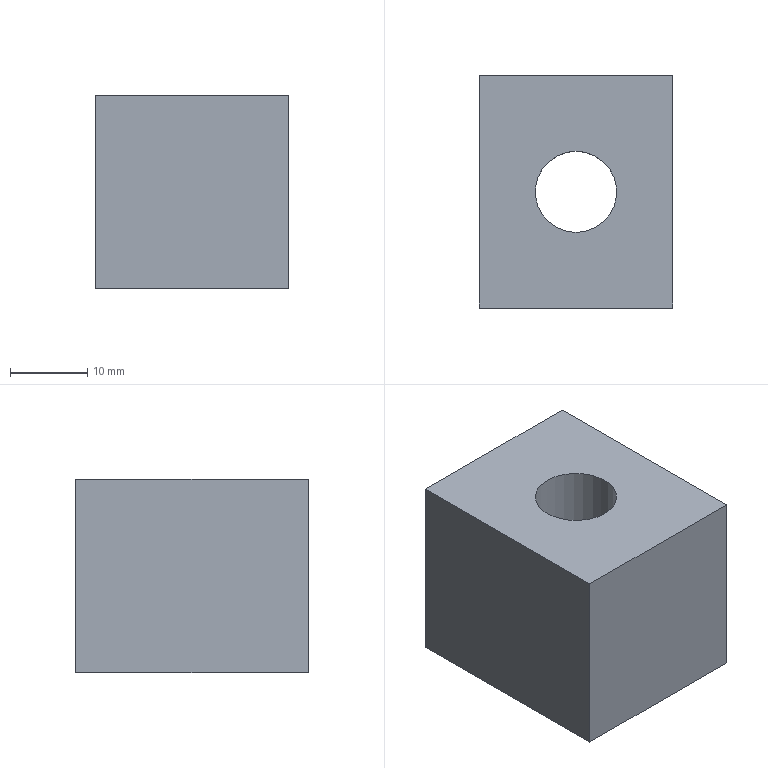Part | STEP file | 1_id1234_x_t | 1 solid | 9 faces | box 25 x 30 x 25 mm | volume 14479 mm3 | plane 7 | cylinder 2 | commonest cylinder face diameters 10.5 x1 17 x1
STEP:
#1=CARTESIAN_POINT('',(0.,0.,0.));
#2=DIRECTION('',(0.,0.,1.));
#3=DIRECTION('',(1.,0.,0.));
#4=AXIS2_PLACEMENT_3D('',#1,#2,#3);
#5=CARTESIAN_POINT('',(614.7,91.944,103.61));
#6=VERTEX_POINT('',#5);
#7=CARTESIAN_POINT('',(597.7,91.944,103.61));
#8=VERTEX_POINT('',#7);
#9=CARTESIAN_POINT('',(606.2,91.944,103.61));
#10=DIRECTION('',(0.,0.,-1.));
#11=DIRECTION('',(1.,0.,0.));
#12=AXIS2_PLACEMENT_3D('',#9,#10,#11);
#13=CIRCLE('',#12,8.5);
#14=CARTESIAN_POINT('',(606.2,91.944,103.61));
#15=DIRECTION('',(0.,0.,1.));
#16=DIRECTION('',(1.,0.,0.));
#17=AXIS2_PLACEMENT_3D('',#14,#15,#16);
#18=PLANE('',#17);
#19=CARTESIAN_POINT('',(8.5,0.));
#20=CARTESIAN_POINT('',(8.5,-14.722));
#21=CARTESIAN_POINT('',(-4.25,-7.361));
#22=CARTESIAN_POINT('',(-17.,0.));
#23=CARTESIAN_POINT('',(-4.25,7.361));
#24=CARTESIAN_POINT('',(8.5,14.722));
#25=CARTESIAN_POINT('',(8.5,0.));
#26=(BOUNDED_CURVE()B_SPLINE_CURVE(2,(#19,#20,#21,#22,#23,#24,#25),.UNSPECIFIED.,.T.,.F.)B_SPLINE_CURVE_WITH_KNOTS((1,2,2,2,2,1),(-2.094,0.,2.094,4.189,6.283,8.378),.UNSPECIFIED.)CURVE()GEOMETRIC_REPRESENTATION_ITEM()RATIONAL_B_SPLINE_CURVE((1.,0.5,1.,0.5,1.,0.5,1.))REPRESENTATION_ITEM(''));
#27=(GEOMETRIC_REPRESENTATION_CONTEXT(2)PARAMETRIC_REPRESENTATION_CONTEXT()REPRESENTATION_CONTEXT('',''));
#28=DEFINITIONAL_REPRESENTATION('',(#26),#27);
#29=PCURVE('',#18,#28);
#30=CARTESIAN_POINT('',(606.2,91.944,103.61));
#31=DIRECTION('',(0.,0.,1.));
#32=DIRECTION('',(-1.,0.,0.));
#33=AXIS2_PLACEMENT_3D('',#30,#31,#32);
#34=CYLINDRICAL_SURFACE('',#33,8.5);
#35=CARTESIAN_POINT('',(3.142,0.));
#36=DIRECTION('',(-1.,0.));
#37=VECTOR('',#36,1.);
#38=LINE('',#35,#37);
#39=(GEOMETRIC_REPRESENTATION_CONTEXT(2)PARAMETRIC_REPRESENTATION_CONTEXT()REPRESENTATION_CONTEXT('',''));
#40=DEFINITIONAL_REPRESENTATION('',(#38),#39);
#41=PCURVE('',#34,#40);
#42=SURFACE_CURVE('',#13,(#29,#41),.PCURVE_S1.);
#43=EDGE_CURVE('',#6,#8,#42,.T.);
#44=ORIENTED_EDGE('',*,*,#43,.T.);
#45=CARTESIAN_POINT('',(606.2,91.944,103.61));
#46=DIRECTION('',(0.,0.,-1.));
#47=DIRECTION('',(1.,0.,0.));
#48=AXIS2_PLACEMENT_3D('',#45,#46,#47);
#49=CIRCLE('',#48,8.5);
#50=CARTESIAN_POINT('',(8.5,0.));
#51=CARTESIAN_POINT('',(8.5,-14.722));
#52=CARTESIAN_POINT('',(-4.25,-7.361));
#53=CARTESIAN_POINT('',(-17.,0.));
#54=CARTESIAN_POINT('',(-4.25,7.361));
#55=CARTESIAN_POINT('',(8.5,14.722));
#56=CARTESIAN_POINT('',(8.5,0.));
#57=(BOUNDED_CURVE()B_SPLINE_CURVE(2,(#50,#51,#52,#53,#54,#55,#56),.UNSPECIFIED.,.T.,.F.)B_SPLINE_CURVE_WITH_KNOTS((1,2,2,2,2,1),(-2.094,0.,2.094,4.189,6.283,8.378),.UNSPECIFIED.)CURVE()GEOMETRIC_REPRESENTATION_ITEM()RATIONAL_B_SPLINE_CURVE((1.,0.5,1.,0.5,1.,0.5,1.))REPRESENTATION_ITEM(''));
#58=(GEOMETRIC_REPRESENTATION_CONTEXT(2)PARAMETRIC_REPRESENTATION_CONTEXT()REPRESENTATION_CONTEXT('',''));
#59=DEFINITIONAL_REPRESENTATION('',(#57),#58);
#60=PCURVE('',#18,#59);
#61=CARTESIAN_POINT('',(9.425,0.));
#62=DIRECTION('',(-1.,0.));
#63=VECTOR('',#62,1.);
#64=LINE('',#61,#63);
#65=(GEOMETRIC_REPRESENTATION_CONTEXT(2)PARAMETRIC_REPRESENTATION_CONTEXT()REPRESENTATION_CONTEXT('',''));
#66=DEFINITIONAL_REPRESENTATION('',(#64),#65);
#67=PCURVE('',#34,#66);
#68=SURFACE_CURVE('',#49,(#60,#67),.PCURVE_S1.);
#69=EDGE_CURVE('',#8,#6,#68,.T.);
#70=ORIENTED_EDGE('',*,*,#69,.T.);
#71=EDGE_LOOP('',(#44,#70));
#72=FACE_BOUND('',#71,.T.);
#73=CARTESIAN_POINT('',(606.2,86.694,103.61));
#74=VERTEX_POINT('',#73);
#75=CARTESIAN_POINT('',(606.2,97.194,103.61));
#76=VERTEX_POINT('',#75);
#77=CARTESIAN_POINT('',(606.2,91.944,103.61));
#78=DIRECTION('',(0.,0.,1.));
#79=DIRECTION('',(0.,-1.,0.));
#80=AXIS2_PLACEMENT_3D('',#77,#78,#79);
#81=CIRCLE('',#80,5.25);
#82=CARTESIAN_POINT('',(0.,0.));
#83=DIRECTION('',(0.,-1.));
#84=AXIS2_PLACEMENT_2D('',#82,#83);
#85=CIRCLE('',#84,5.25);
#86=(GEOMETRIC_REPRESENTATION_CONTEXT(2)PARAMETRIC_REPRESENTATION_CONTEXT()REPRESENTATION_CONTEXT('',''));
#87=DEFINITIONAL_REPRESENTATION('',(#85),#86);
#88=PCURVE('',#18,#87);
#89=CARTESIAN_POINT('',(606.2,91.944,113.86));
#90=DIRECTION('',(0.,0.,1.));
#91=DIRECTION('',(-1.,0.,0.));
#92=AXIS2_PLACEMENT_3D('',#89,#90,#91);
#93=CYLINDRICAL_SURFACE('',#92,5.25);
#94=CARTESIAN_POINT('',(7.854,-10.25));
#95=DIRECTION('',(1.,0.));
#96=VECTOR('',#95,1.);
#97=LINE('',#94,#96);
#98=(GEOMETRIC_REPRESENTATION_CONTEXT(2)PARAMETRIC_REPRESENTATION_CONTEXT()REPRESENTATION_CONTEXT('',''));
#99=DEFINITIONAL_REPRESENTATION('',(#97),#98);
#100=PCURVE('',#93,#99);
#101=SURFACE_CURVE('',#81,(#88,#100),.PCURVE_S1.);
#102=EDGE_CURVE('',#74,#76,#101,.T.);
#103=ORIENTED_EDGE('',*,*,#102,.T.);
#104=CARTESIAN_POINT('',(606.2,91.944,103.61));
#105=DIRECTION('',(0.,0.,1.));
#106=DIRECTION('',(0.,-1.,0.));
#107=AXIS2_PLACEMENT_3D('',#104,#105,#106);
#108=CIRCLE('',#107,5.25);
#109=CARTESIAN_POINT('',(0.,0.));
#110=DIRECTION('',(0.,-1.));
#111=AXIS2_PLACEMENT_2D('',#109,#110);
#112=CIRCLE('',#111,5.25);
#113=(GEOMETRIC_REPRESENTATION_CONTEXT(2)PARAMETRIC_REPRESENTATION_CONTEXT()REPRESENTATION_CONTEXT('',''));
#114=DEFINITIONAL_REPRESENTATION('',(#112),#113);
#115=PCURVE('',#18,#114);
#116=CARTESIAN_POINT('',(1.571,-10.25));
#117=DIRECTION('',(1.,0.));
#118=VECTOR('',#117,1.);
#119=LINE('',#116,#118);
#120=(GEOMETRIC_REPRESENTATION_CONTEXT(2)PARAMETRIC_REPRESENTATION_CONTEXT()REPRESENTATION_CONTEXT('',''));
#121=DEFINITIONAL_REPRESENTATION('',(#119),#120);
#122=PCURVE('',#93,#121);
#123=SURFACE_CURVE('',#108,(#115,#122),.PCURVE_S1.);
#124=EDGE_CURVE('',#76,#74,#123,.T.);
#125=ORIENTED_EDGE('',*,*,#124,.T.);
#126=EDGE_LOOP('',(#103,#125));
#127=FACE_BOUND('',#126,.T.);
#128=ADVANCED_FACE('',(#72,#127),#18,.F.);
#129=ORIENTED_EDGE('',*,*,#43,.T.);
#130=CARTESIAN_POINT('',(597.7,91.944,88.61));
#131=VERTEX_POINT('',#130);
#132=CARTESIAN_POINT('',(597.7,91.944,88.61));
#133=CARTESIAN_POINT('',(597.7,91.944,103.61));
#134=B_SPLINE_CURVE_WITH_KNOTS('',1,(#132,#133),.UNSPECIFIED.,.F.,.F.,(2,2),(-15.,0.),.PIECEWISE_BEZIER_KNOTS.);
#135=CARTESIAN_POINT('',(0.,0.));
#136=DIRECTION('',(0.,1.));
#137=VECTOR('',#136,1.);
#138=LINE('',#135,#137);
#139=(GEOMETRIC_REPRESENTATION_CONTEXT(2)PARAMETRIC_REPRESENTATION_CONTEXT()REPRESENTATION_CONTEXT('',''));
#140=DEFINITIONAL_REPRESENTATION('',(#138),#139);
#141=PCURVE('',#34,#140);
#142=CARTESIAN_POINT('',(6.283,0.));
#143=DIRECTION('',(0.,1.));
#144=VECTOR('',#143,1.);
#145=LINE('',#142,#144);
#146=(GEOMETRIC_REPRESENTATION_CONTEXT(2)PARAMETRIC_REPRESENTATION_CONTEXT()REPRESENTATION_CONTEXT('',''));
#147=DEFINITIONAL_REPRESENTATION('',(#145),#146);
#148=PCURVE('',#34,#147);
#149=SEAM_CURVE('',#134,(#141,#148),.PCURVE_S1.);
#150=EDGE_CURVE('',#131,#8,#149,.T.);
#151=ORIENTED_EDGE('',*,*,#150,.F.);
#152=CARTESIAN_POINT('',(606.2,91.944,88.61));
#153=DIRECTION('',(0.,0.,1.));
#154=DIRECTION('',(-1.,0.,0.));
#155=AXIS2_PLACEMENT_3D('',#152,#153,#154);
#156=CIRCLE('',#155,8.5);
#157=CARTESIAN_POINT('',(0.,-15.));
#158=DIRECTION('',(1.,0.));
#159=VECTOR('',#158,1.);
#160=LINE('',#157,#159);
#161=(GEOMETRIC_REPRESENTATION_CONTEXT(2)PARAMETRIC_REPRESENTATION_CONTEXT()REPRESENTATION_CONTEXT('',''));
#162=DEFINITIONAL_REPRESENTATION('',(#160),#161);
#163=PCURVE('',#34,#162);
#164=CARTESIAN_POINT('',(593.7,26.944,88.61));
#165=DIRECTION('',(0.,0.,-1.));
#166=DIRECTION('',(0.,-1.,0.));
#167=AXIS2_PLACEMENT_3D('',#164,#165,#166);
#168=PLANE('',#167);
#169=CARTESIAN_POINT('',(-65.,-4.));
#170=CARTESIAN_POINT('',(-50.278,-4.));
#171=CARTESIAN_POINT('',(-57.639,-16.75));
#172=CARTESIAN_POINT('',(-65.,-29.5));
#173=CARTESIAN_POINT('',(-72.361,-16.75));
#174=CARTESIAN_POINT('',(-79.722,-4.));
#175=CARTESIAN_POINT('',(-65.,-4.));
#176=(BOUNDED_CURVE()B_SPLINE_CURVE(2,(#169,#170,#171,#172,#173,#174,#175),.UNSPECIFIED.,.T.,.F.)B_SPLINE_CURVE_WITH_KNOTS((1,2,2,2,2,1),(-2.094,0.,2.094,4.189,6.283,8.378),.UNSPECIFIED.)CURVE()GEOMETRIC_REPRESENTATION_ITEM()RATIONAL_B_SPLINE_CURVE((1.,0.5,1.,0.5,1.,0.5,1.))REPRESENTATION_ITEM(''));
#177=(GEOMETRIC_REPRESENTATION_CONTEXT(2)PARAMETRIC_REPRESENTATION_CONTEXT()REPRESENTATION_CONTEXT('',''));
#178=DEFINITIONAL_REPRESENTATION('',(#176),#177);
#179=PCURVE('',#168,#178);
#180=SURFACE_CURVE('',#156,(#163,#179),.PCURVE_S1.);
#181=EDGE_CURVE('',#131,#131,#180,.T.);
#182=ORIENTED_EDGE('',*,*,#181,.T.);
#183=ORIENTED_EDGE('',*,*,#150,.T.);
#184=ORIENTED_EDGE('',*,*,#69,.T.);
#185=EDGE_LOOP('',(#129,#151,#182,#183,#184));
#186=FACE_BOUND('',#185,.F.);
#187=ADVANCED_FACE('',(#186),#34,.F.);
#188=CARTESIAN_POINT('',(593.7,106.944,88.61));
#189=VERTEX_POINT('',#188);
#190=CARTESIAN_POINT('',(593.7,76.944,88.61));
#191=VERTEX_POINT('',#190);
#192=CARTESIAN_POINT('',(593.7,106.944,88.61));
#193=DIRECTION('',(0.,-1.,0.));
#194=VECTOR('',#193,1.);
#195=LINE('',#192,#194);
#196=CARTESIAN_POINT('',(-80.,0.));
#197=DIRECTION('',(1.,0.));
#198=VECTOR('',#197,1.);
#199=LINE('',#196,#198);
#200=(GEOMETRIC_REPRESENTATION_CONTEXT(2)PARAMETRIC_REPRESENTATION_CONTEXT()REPRESENTATION_CONTEXT('',''));
#201=DEFINITIONAL_REPRESENTATION('',(#199),#200);
#202=PCURVE('',#168,#201);
#203=CARTESIAN_POINT('',(593.7,26.944,113.61));
#204=DIRECTION('',(-1.,0.,0.));
#205=DIRECTION('',(0.,0.,-1.));
#206=AXIS2_PLACEMENT_3D('',#203,#204,#205);
#207=PLANE('',#206);
#208=CARTESIAN_POINT('',(25.,-80.));
#209=DIRECTION('',(0.,1.));
#210=VECTOR('',#209,1.);
#211=LINE('',#208,#210);
#212=(GEOMETRIC_REPRESENTATION_CONTEXT(2)PARAMETRIC_REPRESENTATION_CONTEXT()REPRESENTATION_CONTEXT('',''));
#213=DEFINITIONAL_REPRESENTATION('',(#211),#212);
#214=PCURVE('',#207,#213);
#215=SURFACE_CURVE('',#195,(#202,#214),.PCURVE_S1.);
#216=EDGE_CURVE('',#189,#191,#215,.T.);
#217=ORIENTED_EDGE('',*,*,#216,.F.);
#218=CARTESIAN_POINT('',(618.7,106.944,88.61));
#219=VERTEX_POINT('',#218);
#220=CARTESIAN_POINT('',(618.7,106.944,88.61));
#221=DIRECTION('',(-1.,0.,0.));
#222=VECTOR('',#221,1.);
#223=LINE('',#220,#222);
#224=CARTESIAN_POINT('',(-80.,-25.));
#225=DIRECTION('',(0.,1.));
#226=VECTOR('',#225,1.);
#227=LINE('',#224,#226);
#228=(GEOMETRIC_REPRESENTATION_CONTEXT(2)PARAMETRIC_REPRESENTATION_CONTEXT()REPRESENTATION_CONTEXT('',''));
#229=DEFINITIONAL_REPRESENTATION('',(#227),#228);
#230=PCURVE('',#168,#229);
#231=CARTESIAN_POINT('',(593.7,106.944,113.61));
#232=DIRECTION('',(0.,1.,0.));
#233=DIRECTION('',(-1.,0.,0.));
#234=AXIS2_PLACEMENT_3D('',#231,#232,#233);
#235=PLANE('',#234);
#236=CARTESIAN_POINT('',(-25.,-25.));
#237=DIRECTION('',(1.,0.));
#238=VECTOR('',#237,1.);
#239=LINE('',#236,#238);
#240=(GEOMETRIC_REPRESENTATION_CONTEXT(2)PARAMETRIC_REPRESENTATION_CONTEXT()REPRESENTATION_CONTEXT('',''));
#241=DEFINITIONAL_REPRESENTATION('',(#239),#240);
#242=PCURVE('',#235,#241);
#243=SURFACE_CURVE('',#223,(#230,#242),.PCURVE_S1.);
#244=EDGE_CURVE('',#219,#189,#243,.T.);
#245=ORIENTED_EDGE('',*,*,#244,.F.);
#246=CARTESIAN_POINT('',(618.7,76.944,88.61));
#247=VERTEX_POINT('',#246);
#248=CARTESIAN_POINT('',(618.7,76.944,88.61));
#249=DIRECTION('',(0.,1.,0.));
#250=VECTOR('',#249,1.);
#251=LINE('',#248,#250);
#252=CARTESIAN_POINT('',(-50.,-25.));
#253=DIRECTION('',(-1.,0.));
#254=VECTOR('',#253,1.);
#255=LINE('',#252,#254);
#256=(GEOMETRIC_REPRESENTATION_CONTEXT(2)PARAMETRIC_REPRESENTATION_CONTEXT()REPRESENTATION_CONTEXT('',''));
#257=DEFINITIONAL_REPRESENTATION('',(#255),#256);
#258=PCURVE('',#168,#257);
#259=CARTESIAN_POINT('',(618.7,106.944,113.61));
#260=DIRECTION('',(1.,0.,0.));
#261=DIRECTION('',(0.,-1.,0.));
#262=AXIS2_PLACEMENT_3D('',#259,#260,#261);
#263=PLANE('',#262);
#264=CARTESIAN_POINT('',(30.,25.));
#265=DIRECTION('',(-1.,0.));
#266=VECTOR('',#265,1.);
#267=LINE('',#264,#266);
#268=(GEOMETRIC_REPRESENTATION_CONTEXT(2)PARAMETRIC_REPRESENTATION_CONTEXT()REPRESENTATION_CONTEXT('',''));
#269=DEFINITIONAL_REPRESENTATION('',(#267),#268);
#270=PCURVE('',#263,#269);
#271=SURFACE_CURVE('',#251,(#258,#270),.PCURVE_S1.);
#272=EDGE_CURVE('',#247,#219,#271,.T.);
#273=ORIENTED_EDGE('',*,*,#272,.F.);
#274=CARTESIAN_POINT('',(618.7,76.944,88.61));
#275=DIRECTION('',(-1.,0.,0.));
#276=VECTOR('',#275,1.);
#277=LINE('',#274,#276);
#278=CARTESIAN_POINT('',(-50.,-25.));
#279=DIRECTION('',(0.,1.));
#280=VECTOR('',#279,1.);
#281=LINE('',#278,#280);
#282=(GEOMETRIC_REPRESENTATION_CONTEXT(2)PARAMETRIC_REPRESENTATION_CONTEXT()REPRESENTATION_CONTEXT('',''));
#283=DEFINITIONAL_REPRESENTATION('',(#281),#282);
#284=PCURVE('',#168,#283);
#285=CARTESIAN_POINT('',(606.2,76.944,100.935));
#286=DIRECTION('',(0.,1.,0.));
#287=DIRECTION('',(0.,0.,1.));
#288=AXIS2_PLACEMENT_3D('',#285,#286,#287);
#289=PLANE('',#288);
#290=CARTESIAN_POINT('',(-12.325,12.5));
#291=DIRECTION('',(0.,-1.));
#292=VECTOR('',#291,1.);
#293=LINE('',#290,#292);
#294=(GEOMETRIC_REPRESENTATION_CONTEXT(2)PARAMETRIC_REPRESENTATION_CONTEXT()REPRESENTATION_CONTEXT('',''));
#295=DEFINITIONAL_REPRESENTATION('',(#293),#294);
#296=PCURVE('',#289,#295);
#297=SURFACE_CURVE('',#277,(#284,#296),.PCURVE_S1.);
#298=EDGE_CURVE('',#247,#191,#297,.T.);
#299=ORIENTED_EDGE('',*,*,#298,.T.);
#300=EDGE_LOOP('',(#217,#245,#273,#299));
#301=FACE_BOUND('',#300,.T.);
#302=ORIENTED_EDGE('',*,*,#181,.T.);
#303=EDGE_LOOP('',(#302));
#304=FACE_BOUND('',#303,.T.);
#305=ADVANCED_FACE('',(#301,#304),#168,.T.);
#306=CARTESIAN_POINT('',(618.7,76.944,113.61));
#307=VERTEX_POINT('',#306);
#308=CARTESIAN_POINT('',(618.7,76.944,113.61));
#309=DIRECTION('',(0.,0.,-1.));
#310=VECTOR('',#309,1.);
#311=LINE('',#308,#310);
#312=CARTESIAN_POINT('',(12.675,12.5));
#313=DIRECTION('',(-1.,0.));
#314=VECTOR('',#313,1.);
#315=LINE('',#312,#314);
#316=(GEOMETRIC_REPRESENTATION_CONTEXT(2)PARAMETRIC_REPRESENTATION_CONTEXT()REPRESENTATION_CONTEXT('',''));
#317=DEFINITIONAL_REPRESENTATION('',(#315),#316);
#318=PCURVE('',#289,#317);
#319=CARTESIAN_POINT('',(30.,0.));
#320=DIRECTION('',(0.,1.));
#321=VECTOR('',#320,1.);
#322=LINE('',#319,#321);
#323=(GEOMETRIC_REPRESENTATION_CONTEXT(2)PARAMETRIC_REPRESENTATION_CONTEXT()REPRESENTATION_CONTEXT('',''));
#324=DEFINITIONAL_REPRESENTATION('',(#322),#323);
#325=PCURVE('',#263,#324);
#326=SURFACE_CURVE('',#311,(#318,#325),.PCURVE_S1.);
#327=EDGE_CURVE('',#307,#247,#326,.T.);
#328=ORIENTED_EDGE('',*,*,#327,.F.);
#329=CARTESIAN_POINT('',(593.7,76.944,113.61));
#330=VERTEX_POINT('',#329);
#331=CARTESIAN_POINT('',(618.7,76.944,113.61));
#332=DIRECTION('',(-1.,0.,0.));
#333=VECTOR('',#332,1.);
#334=LINE('',#331,#333);
#335=CARTESIAN_POINT('',(12.675,12.5));
#336=DIRECTION('',(0.,-1.));
#337=VECTOR('',#336,1.);
#338=LINE('',#335,#337);
#339=(GEOMETRIC_REPRESENTATION_CONTEXT(2)PARAMETRIC_REPRESENTATION_CONTEXT()REPRESENTATION_CONTEXT('',''));
#340=DEFINITIONAL_REPRESENTATION('',(#338),#339);
#341=PCURVE('',#289,#340);
#342=CARTESIAN_POINT('',(593.7,26.944,113.61));
#343=DIRECTION('',(0.,0.,-1.));
#344=DIRECTION('',(0.,-1.,0.));
#345=AXIS2_PLACEMENT_3D('',#342,#343,#344);
#346=PLANE('',#345);
#347=CARTESIAN_POINT('',(-50.,-25.));
#348=DIRECTION('',(0.,1.));
#349=VECTOR('',#348,1.);
#350=LINE('',#347,#349);
#351=(GEOMETRIC_REPRESENTATION_CONTEXT(2)PARAMETRIC_REPRESENTATION_CONTEXT()REPRESENTATION_CONTEXT('',''));
#352=DEFINITIONAL_REPRESENTATION('',(#350),#351);
#353=PCURVE('',#346,#352);
#354=SURFACE_CURVE('',#334,(#341,#353),.PCURVE_S1.);
#355=EDGE_CURVE('',#307,#330,#354,.T.);
#356=ORIENTED_EDGE('',*,*,#355,.T.);
#357=CARTESIAN_POINT('',(593.7,76.944,88.61));
#358=DIRECTION('',(0.,0.,1.));
#359=VECTOR('',#358,1.);
#360=LINE('',#357,#359);
#361=CARTESIAN_POINT('',(-12.325,-12.5));
#362=DIRECTION('',(1.,0.));
#363=VECTOR('',#362,1.);
#364=LINE('',#361,#363);
#365=(GEOMETRIC_REPRESENTATION_CONTEXT(2)PARAMETRIC_REPRESENTATION_CONTEXT()REPRESENTATION_CONTEXT('',''));
#366=DEFINITIONAL_REPRESENTATION('',(#364),#365);
#367=PCURVE('',#289,#366);
#368=CARTESIAN_POINT('',(25.,-50.));
#369=DIRECTION('',(-1.,0.));
#370=VECTOR('',#369,1.);
#371=LINE('',#368,#370);
#372=(GEOMETRIC_REPRESENTATION_CONTEXT(2)PARAMETRIC_REPRESENTATION_CONTEXT()REPRESENTATION_CONTEXT('',''));
#373=DEFINITIONAL_REPRESENTATION('',(#371),#372);
#374=PCURVE('',#207,#373);
#375=SURFACE_CURVE('',#360,(#367,#374),.PCURVE_S1.);
#376=EDGE_CURVE('',#191,#330,#375,.T.);
#377=ORIENTED_EDGE('',*,*,#376,.F.);
#378=ORIENTED_EDGE('',*,*,#298,.F.);
#379=EDGE_LOOP('',(#328,#356,#377,#378));
#380=FACE_BOUND('',#379,.T.);
#381=ADVANCED_FACE('',(#380),#289,.F.);
#382=CARTESIAN_POINT('',(593.7,106.944,113.61));
#383=VERTEX_POINT('',#382);
#384=CARTESIAN_POINT('',(593.7,106.944,113.61));
#385=DIRECTION('',(0.,-1.,0.));
#386=VECTOR('',#385,1.);
#387=LINE('',#384,#386);
#388=CARTESIAN_POINT('',(0.,-80.));
#389=DIRECTION('',(0.,1.));
#390=VECTOR('',#389,1.);
#391=LINE('',#388,#390);
#392=(GEOMETRIC_REPRESENTATION_CONTEXT(2)PARAMETRIC_REPRESENTATION_CONTEXT()REPRESENTATION_CONTEXT('',''));
#393=DEFINITIONAL_REPRESENTATION('',(#391),#392);
#394=PCURVE('',#207,#393);
#395=CARTESIAN_POINT('',(-80.,0.));
#396=DIRECTION('',(1.,0.));
#397=VECTOR('',#396,1.);
#398=LINE('',#395,#397);
#399=(GEOMETRIC_REPRESENTATION_CONTEXT(2)PARAMETRIC_REPRESENTATION_CONTEXT()REPRESENTATION_CONTEXT('',''));
#400=DEFINITIONAL_REPRESENTATION('',(#398),#399);
#401=PCURVE('',#346,#400);
#402=SURFACE_CURVE('',#387,(#394,#401),.PCURVE_S1.);
#403=EDGE_CURVE('',#383,#330,#402,.T.);
#404=ORIENTED_EDGE('',*,*,#403,.F.);
#405=CARTESIAN_POINT('',(593.7,106.944,88.61));
#406=DIRECTION('',(0.,0.,1.));
#407=VECTOR('',#406,1.);
#408=LINE('',#405,#407);
#409=CARTESIAN_POINT('',(25.,-80.));
#410=DIRECTION('',(-1.,0.));
#411=VECTOR('',#410,1.);
#412=LINE('',#409,#411);
#413=(GEOMETRIC_REPRESENTATION_CONTEXT(2)PARAMETRIC_REPRESENTATION_CONTEXT()REPRESENTATION_CONTEXT('',''));
#414=DEFINITIONAL_REPRESENTATION('',(#412),#413);
#415=PCURVE('',#207,#414);
#416=CARTESIAN_POINT('',(0.,-25.));
#417=DIRECTION('',(0.,1.));
#418=VECTOR('',#417,1.);
#419=LINE('',#416,#418);
#420=(GEOMETRIC_REPRESENTATION_CONTEXT(2)PARAMETRIC_REPRESENTATION_CONTEXT()REPRESENTATION_CONTEXT('',''));
#421=DEFINITIONAL_REPRESENTATION('',(#419),#420);
#422=PCURVE('',#235,#421);
#423=SURFACE_CURVE('',#408,(#415,#422),.PCURVE_S1.);
#424=EDGE_CURVE('',#189,#383,#423,.T.);
#425=ORIENTED_EDGE('',*,*,#424,.F.);
#426=ORIENTED_EDGE('',*,*,#216,.T.);
#427=ORIENTED_EDGE('',*,*,#376,.T.);
#428=EDGE_LOOP('',(#404,#425,#426,#427));
#429=FACE_BOUND('',#428,.T.);
#430=ADVANCED_FACE('',(#429),#207,.T.);
#431=ORIENTED_EDGE('',*,*,#424,.T.);
#432=CARTESIAN_POINT('',(618.7,106.944,113.61));
#433=VERTEX_POINT('',#432);
#434=CARTESIAN_POINT('',(618.7,106.944,113.61));
#435=DIRECTION('',(-1.,0.,0.));
#436=VECTOR('',#435,1.);
#437=LINE('',#434,#436);
#438=CARTESIAN_POINT('',(-25.,0.));
#439=DIRECTION('',(1.,0.));
#440=VECTOR('',#439,1.);
#441=LINE('',#438,#440);
#442=(GEOMETRIC_REPRESENTATION_CONTEXT(2)PARAMETRIC_REPRESENTATION_CONTEXT()REPRESENTATION_CONTEXT('',''));
#443=DEFINITIONAL_REPRESENTATION('',(#441),#442);
#444=PCURVE('',#235,#443);
#445=CARTESIAN_POINT('',(-80.,-25.));
#446=DIRECTION('',(0.,1.));
#447=VECTOR('',#446,1.);
#448=LINE('',#445,#447);
#449=(GEOMETRIC_REPRESENTATION_CONTEXT(2)PARAMETRIC_REPRESENTATION_CONTEXT()REPRESENTATION_CONTEXT('',''));
#450=DEFINITIONAL_REPRESENTATION('',(#448),#449);
#451=PCURVE('',#346,#450);
#452=SURFACE_CURVE('',#437,(#444,#451),.PCURVE_S1.);
#453=EDGE_CURVE('',#433,#383,#452,.T.);
#454=ORIENTED_EDGE('',*,*,#453,.F.);
#455=CARTESIAN_POINT('',(618.7,106.944,88.61));
#456=DIRECTION('',(0.,0.,1.));
#457=VECTOR('',#456,1.);
#458=LINE('',#455,#457);
#459=CARTESIAN_POINT('',(-25.,-25.));
#460=DIRECTION('',(0.,1.));
#461=VECTOR('',#460,1.);
#462=LINE('',#459,#461);
#463=(GEOMETRIC_REPRESENTATION_CONTEXT(2)PARAMETRIC_REPRESENTATION_CONTEXT()REPRESENTATION_CONTEXT('',''));
#464=DEFINITIONAL_REPRESENTATION('',(#462),#463);
#465=PCURVE('',#235,#464);
#466=CARTESIAN_POINT('',(0.,25.));
#467=DIRECTION('',(0.,-1.));
#468=VECTOR('',#467,1.);
#469=LINE('',#466,#468);
#470=(GEOMETRIC_REPRESENTATION_CONTEXT(2)PARAMETRIC_REPRESENTATION_CONTEXT()REPRESENTATION_CONTEXT('',''));
#471=DEFINITIONAL_REPRESENTATION('',(#469),#470);
#472=PCURVE('',#263,#471);
#473=SURFACE_CURVE('',#458,(#465,#472),.PCURVE_S1.);
#474=EDGE_CURVE('',#219,#433,#473,.T.);
#475=ORIENTED_EDGE('',*,*,#474,.F.);
#476=ORIENTED_EDGE('',*,*,#244,.T.);
#477=EDGE_LOOP('',(#431,#454,#475,#476));
#478=FACE_BOUND('',#477,.T.);
#479=ADVANCED_FACE('',(#478),#235,.T.);
#480=ORIENTED_EDGE('',*,*,#272,.T.);
#481=ORIENTED_EDGE('',*,*,#474,.T.);
#482=CARTESIAN_POINT('',(618.7,76.944,113.61));
#483=DIRECTION('',(0.,1.,0.));
#484=VECTOR('',#483,1.);
#485=LINE('',#482,#484);
#486=CARTESIAN_POINT('',(30.,0.));
#487=DIRECTION('',(-1.,0.));
#488=VECTOR('',#487,1.);
#489=LINE('',#486,#488);
#490=(GEOMETRIC_REPRESENTATION_CONTEXT(2)PARAMETRIC_REPRESENTATION_CONTEXT()REPRESENTATION_CONTEXT('',''));
#491=DEFINITIONAL_REPRESENTATION('',(#489),#490);
#492=PCURVE('',#263,#491);
#493=CARTESIAN_POINT('',(-50.,-25.));
#494=DIRECTION('',(-1.,0.));
#495=VECTOR('',#494,1.);
#496=LINE('',#493,#495);
#497=(GEOMETRIC_REPRESENTATION_CONTEXT(2)PARAMETRIC_REPRESENTATION_CONTEXT()REPRESENTATION_CONTEXT('',''));
#498=DEFINITIONAL_REPRESENTATION('',(#496),#497);
#499=PCURVE('',#346,#498);
#500=SURFACE_CURVE('',#485,(#492,#499),.PCURVE_S1.);
#501=EDGE_CURVE('',#307,#433,#500,.T.);
#502=ORIENTED_EDGE('',*,*,#501,.F.);
#503=ORIENTED_EDGE('',*,*,#327,.T.);
#504=EDGE_LOOP('',(#480,#481,#502,#503));
#505=FACE_BOUND('',#504,.T.);
#506=ADVANCED_FACE('',(#505),#263,.T.);
#507=ORIENTED_EDGE('',*,*,#355,.F.);
#508=ORIENTED_EDGE('',*,*,#501,.T.);
#509=ORIENTED_EDGE('',*,*,#453,.T.);
#510=ORIENTED_EDGE('',*,*,#403,.T.);
#511=EDGE_LOOP('',(#507,#508,#509,#510));
#512=FACE_BOUND('',#511,.T.);
#513=CARTESIAN_POINT('',(606.2,97.194,113.61));
#514=VERTEX_POINT('',#513);
#515=CARTESIAN_POINT('',(606.2,91.944,113.61));
#516=DIRECTION('',(0.,0.,-1.));
#517=DIRECTION('',(0.,1.,0.));
#518=AXIS2_PLACEMENT_3D('',#515,#516,#517);
#519=CIRCLE('',#518,5.25);
#520=CARTESIAN_POINT('',(-65.,-12.5));
#521=DIRECTION('',(-1.,0.));
#522=AXIS2_PLACEMENT_2D('',#520,#521);
#523=CIRCLE('',#522,5.25);
#524=(GEOMETRIC_REPRESENTATION_CONTEXT(2)PARAMETRIC_REPRESENTATION_CONTEXT()REPRESENTATION_CONTEXT('',''));
#525=DEFINITIONAL_REPRESENTATION('',(#523),#524);
#526=PCURVE('',#346,#525);
#527=CARTESIAN_POINT('',(10.996,-0.25));
#528=DIRECTION('',(-1.,0.));
#529=VECTOR('',#528,1.);
#530=LINE('',#527,#529);
#531=(GEOMETRIC_REPRESENTATION_CONTEXT(2)PARAMETRIC_REPRESENTATION_CONTEXT()REPRESENTATION_CONTEXT('',''));
#532=DEFINITIONAL_REPRESENTATION('',(#530),#531);
#533=PCURVE('',#93,#532);
#534=SURFACE_CURVE('',#519,(#526,#533),.PCURVE_S1.);
#535=EDGE_CURVE('',#514,#514,#534,.T.);
#536=ORIENTED_EDGE('',*,*,#535,.T.);
#537=EDGE_LOOP('',(#536));
#538=FACE_BOUND('',#537,.T.);
#539=ADVANCED_FACE('',(#512,#538),#346,.F.);
#540=ORIENTED_EDGE('',*,*,#535,.T.);
#541=CARTESIAN_POINT('',(606.2,97.194,103.61));
#542=CARTESIAN_POINT('',(606.2,97.194,113.61));
#543=B_SPLINE_CURVE_WITH_KNOTS('',1,(#541,#542),.UNSPECIFIED.,.F.,.F.,(2,2),(-10.25,-0.25),.PIECEWISE_BEZIER_KNOTS.);
#544=CARTESIAN_POINT('',(4.712,0.));
#545=DIRECTION('',(0.,1.));
#546=VECTOR('',#545,1.);
#547=LINE('',#544,#546);
#548=(GEOMETRIC_REPRESENTATION_CONTEXT(2)PARAMETRIC_REPRESENTATION_CONTEXT()REPRESENTATION_CONTEXT('',''));
#549=DEFINITIONAL_REPRESENTATION('',(#547),#548);
#550=PCURVE('',#93,#549);
#551=CARTESIAN_POINT('',(10.996,0.));
#552=DIRECTION('',(0.,1.));
#553=VECTOR('',#552,1.);
#554=LINE('',#551,#553);
#555=(GEOMETRIC_REPRESENTATION_CONTEXT(2)PARAMETRIC_REPRESENTATION_CONTEXT()REPRESENTATION_CONTEXT('',''));
#556=DEFINITIONAL_REPRESENTATION('',(#554),#555);
#557=PCURVE('',#93,#556);
#558=SEAM_CURVE('',#543,(#550,#557),.PCURVE_S1.);
#559=EDGE_CURVE('',#76,#514,#558,.T.);
#560=ORIENTED_EDGE('',*,*,#559,.F.);
#561=ORIENTED_EDGE('',*,*,#124,.T.);
#562=ORIENTED_EDGE('',*,*,#102,.T.);
#563=ORIENTED_EDGE('',*,*,#559,.T.);
#564=EDGE_LOOP('',(#540,#560,#561,#562,#563));
#565=FACE_BOUND('',#564,.F.);
#566=ADVANCED_FACE('',(#565),#93,.F.);
#567=CLOSED_SHELL('',(#128,#187,#305,#381,#430,#479,#506,#539,#566));
#568=MANIFOLD_SOLID_BREP('',#567);
#569=(LENGTH_UNIT()NAMED_UNIT(*)SI_UNIT(.MILLI.,.METRE.));
#570=UNCERTAINTY_MEASURE_WITH_UNIT(LENGTH_MEASURE(0.000002),#569,'','');
#571=(NAMED_UNIT(*)PLANE_ANGLE_UNIT()SI_UNIT($,.RADIAN.));
#572=(NAMED_UNIT(*)SI_UNIT($,.STERADIAN.)SOLID_ANGLE_UNIT());
#573=(GEOMETRIC_REPRESENTATION_CONTEXT(3)GLOBAL_UNCERTAINTY_ASSIGNED_CONTEXT((#570))GLOBAL_UNIT_ASSIGNED_CONTEXT((#569,#571,#572))REPRESENTATION_CONTEXT('',''));
#574=ADVANCED_BREP_SHAPE_REPRESENTATION('',(#4,#568),#573);